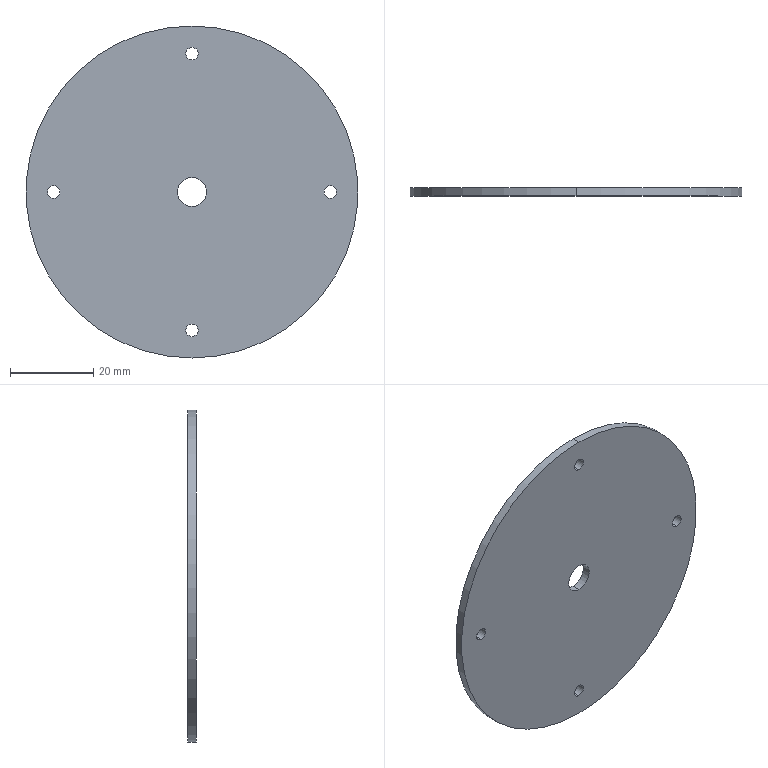Part | SolidWorks | features Cut 2, Extrusion 1 | 1 solid | 14 faces | box 80 x 2 x 80 mm | volume 9920 mm3 | cylinder 12 | plane 2 | commonest cylinder face diameters 3 x8 7 x2 80 x2
STEP:
#1=CARTESIAN_POINT('',(0.,0.,-34.839));
#2=VERTEX_POINT('',#1);
#3=CARTESIAN_POINT('',(0.,0.,-31.839));
#4=VERTEX_POINT('',#3);
#5=CARTESIAN_POINT('',(0.,0.,-33.339));
#6=DIRECTION('',(0.,1.,0.));
#7=DIRECTION('',(0.,0.,1.));
#8=AXIS2_PLACEMENT_3D('',#5,#6,#7);
#9=CIRCLE('',#8,1.5);
#10=EDGE_CURVE('',#2,#4,#9,.T.);
#11=ORIENTED_EDGE('',*,*,#10,.F.);
#12=CARTESIAN_POINT('',(0.,2.,-34.839));
#13=VERTEX_POINT('',#12);
#14=CARTESIAN_POINT('',(0.,-43.,-34.839));
#15=DIRECTION('',(0.,1.,0.));
#16=VECTOR('',#15,1000.);
#17=LINE('',#14,#16);
#18=EDGE_CURVE('',#2,#13,#17,.T.);
#19=ORIENTED_EDGE('',*,*,#18,.T.);
#20=CARTESIAN_POINT('',(0.,2.,-31.839));
#21=VERTEX_POINT('',#20);
#22=CARTESIAN_POINT('',(0.,2.,-33.339));
#23=DIRECTION('',(0.,1.,0.));
#24=DIRECTION('',(0.,0.,1.));
#25=AXIS2_PLACEMENT_3D('',#22,#23,#24);
#26=CIRCLE('',#25,1.5);
#27=EDGE_CURVE('',#13,#21,#26,.T.);
#28=ORIENTED_EDGE('',*,*,#27,.T.);
#29=CARTESIAN_POINT('',(0.,-43.,-31.839));
#30=DIRECTION('',(0.,1.,0.));
#31=VECTOR('',#30,1000.);
#32=LINE('',#29,#31);
#33=EDGE_CURVE('',#4,#21,#32,.T.);
#34=ORIENTED_EDGE('',*,*,#33,.F.);
#35=EDGE_LOOP('',(#11,#19,#28,#34));
#36=FACE_OUTER_BOUND('',#35,.T.);
#37=CARTESIAN_POINT('',(0.,-43.,-33.339));
#38=DIRECTION('',(0.,1.,0.));
#39=DIRECTION('',(0.,0.,1.));
#40=AXIS2_PLACEMENT_3D('',#37,#38,#39);
#41=CYLINDRICAL_SURFACE('',#40,1.5);
#42=ADVANCED_FACE('',(#36),#41,.F.);
#43=CARTESIAN_POINT('',(33.339,0.,-1.5));
#44=VERTEX_POINT('',#43);
#45=CARTESIAN_POINT('',(33.339,0.,1.5));
#46=VERTEX_POINT('',#45);
#47=CARTESIAN_POINT('',(33.339,0.,0.));
#48=DIRECTION('',(0.,1.,0.));
#49=DIRECTION('',(0.,0.,1.));
#50=AXIS2_PLACEMENT_3D('',#47,#48,#49);
#51=CIRCLE('',#50,1.5);
#52=EDGE_CURVE('',#44,#46,#51,.T.);
#53=ORIENTED_EDGE('',*,*,#52,.F.);
#54=CARTESIAN_POINT('',(33.339,2.,-1.5));
#55=VERTEX_POINT('',#54);
#56=CARTESIAN_POINT('',(33.339,-43.,-1.5));
#57=DIRECTION('',(0.,1.,0.));
#58=VECTOR('',#57,1000.);
#59=LINE('',#56,#58);
#60=EDGE_CURVE('',#44,#55,#59,.T.);
#61=ORIENTED_EDGE('',*,*,#60,.T.);
#62=CARTESIAN_POINT('',(33.339,2.,1.5));
#63=VERTEX_POINT('',#62);
#64=CARTESIAN_POINT('',(33.339,2.,0.));
#65=DIRECTION('',(0.,1.,0.));
#66=DIRECTION('',(0.,0.,1.));
#67=AXIS2_PLACEMENT_3D('',#64,#65,#66);
#68=CIRCLE('',#67,1.5);
#69=EDGE_CURVE('',#55,#63,#68,.T.);
#70=ORIENTED_EDGE('',*,*,#69,.T.);
#71=CARTESIAN_POINT('',(33.339,-43.,1.5));
#72=DIRECTION('',(0.,1.,0.));
#73=VECTOR('',#72,1000.);
#74=LINE('',#71,#73);
#75=EDGE_CURVE('',#46,#63,#74,.T.);
#76=ORIENTED_EDGE('',*,*,#75,.F.);
#77=EDGE_LOOP('',(#53,#61,#70,#76));
#78=FACE_OUTER_BOUND('',#77,.T.);
#79=CARTESIAN_POINT('',(33.339,-43.,0.));
#80=DIRECTION('',(0.,1.,0.));
#81=DIRECTION('',(0.,0.,1.));
#82=AXIS2_PLACEMENT_3D('',#79,#80,#81);
#83=CYLINDRICAL_SURFACE('',#82,1.5);
#84=ADVANCED_FACE('',(#78),#83,.F.);
#85=CARTESIAN_POINT('',(0.,0.,31.839));
#86=VERTEX_POINT('',#85);
#87=CARTESIAN_POINT('',(0.,0.,34.839));
#88=VERTEX_POINT('',#87);
#89=CARTESIAN_POINT('',(0.,0.,33.339));
#90=DIRECTION('',(0.,1.,0.));
#91=DIRECTION('',(0.,0.,1.));
#92=AXIS2_PLACEMENT_3D('',#89,#90,#91);
#93=CIRCLE('',#92,1.5);
#94=EDGE_CURVE('',#86,#88,#93,.T.);
#95=ORIENTED_EDGE('',*,*,#94,.F.);
#96=CARTESIAN_POINT('',(0.,2.,31.839));
#97=VERTEX_POINT('',#96);
#98=CARTESIAN_POINT('',(0.,-43.,31.839));
#99=DIRECTION('',(0.,1.,0.));
#100=VECTOR('',#99,1000.);
#101=LINE('',#98,#100);
#102=EDGE_CURVE('',#86,#97,#101,.T.);
#103=ORIENTED_EDGE('',*,*,#102,.T.);
#104=CARTESIAN_POINT('',(0.,2.,34.839));
#105=VERTEX_POINT('',#104);
#106=CARTESIAN_POINT('',(0.,2.,33.339));
#107=DIRECTION('',(0.,1.,0.));
#108=DIRECTION('',(0.,0.,1.));
#109=AXIS2_PLACEMENT_3D('',#106,#107,#108);
#110=CIRCLE('',#109,1.5);
#111=EDGE_CURVE('',#97,#105,#110,.T.);
#112=ORIENTED_EDGE('',*,*,#111,.T.);
#113=CARTESIAN_POINT('',(0.,-43.,34.839));
#114=DIRECTION('',(0.,1.,0.));
#115=VECTOR('',#114,1000.);
#116=LINE('',#113,#115);
#117=EDGE_CURVE('',#88,#105,#116,.T.);
#118=ORIENTED_EDGE('',*,*,#117,.F.);
#119=EDGE_LOOP('',(#95,#103,#112,#118));
#120=FACE_OUTER_BOUND('',#119,.T.);
#121=CARTESIAN_POINT('',(0.,-43.,33.339));
#122=DIRECTION('',(0.,1.,0.));
#123=DIRECTION('',(0.,0.,1.));
#124=AXIS2_PLACEMENT_3D('',#121,#122,#123);
#125=CYLINDRICAL_SURFACE('',#124,1.5);
#126=ADVANCED_FACE('',(#120),#125,.F.);
#127=CARTESIAN_POINT('',(-33.339,0.,-1.5));
#128=VERTEX_POINT('',#127);
#129=CARTESIAN_POINT('',(-33.339,0.,1.5));
#130=VERTEX_POINT('',#129);
#131=CARTESIAN_POINT('',(-33.339,0.,0.));
#132=DIRECTION('',(0.,1.,0.));
#133=DIRECTION('',(0.,0.,1.));
#134=AXIS2_PLACEMENT_3D('',#131,#132,#133);
#135=CIRCLE('',#134,1.5);
#136=EDGE_CURVE('',#128,#130,#135,.T.);
#137=ORIENTED_EDGE('',*,*,#136,.F.);
#138=CARTESIAN_POINT('',(-33.339,2.,-1.5));
#139=VERTEX_POINT('',#138);
#140=CARTESIAN_POINT('',(-33.339,-43.,-1.5));
#141=DIRECTION('',(0.,1.,0.));
#142=VECTOR('',#141,1000.);
#143=LINE('',#140,#142);
#144=EDGE_CURVE('',#128,#139,#143,.T.);
#145=ORIENTED_EDGE('',*,*,#144,.T.);
#146=CARTESIAN_POINT('',(-33.339,2.,1.5));
#147=VERTEX_POINT('',#146);
#148=CARTESIAN_POINT('',(-33.339,2.,0.));
#149=DIRECTION('',(0.,1.,0.));
#150=DIRECTION('',(0.,0.,1.));
#151=AXIS2_PLACEMENT_3D('',#148,#149,#150);
#152=CIRCLE('',#151,1.5);
#153=EDGE_CURVE('',#139,#147,#152,.T.);
#154=ORIENTED_EDGE('',*,*,#153,.T.);
#155=CARTESIAN_POINT('',(-33.339,-43.,1.5));
#156=DIRECTION('',(0.,1.,0.));
#157=VECTOR('',#156,1000.);
#158=LINE('',#155,#157);
#159=EDGE_CURVE('',#130,#147,#158,.T.);
#160=ORIENTED_EDGE('',*,*,#159,.F.);
#161=EDGE_LOOP('',(#137,#145,#154,#160));
#162=FACE_OUTER_BOUND('',#161,.T.);
#163=CARTESIAN_POINT('',(-33.339,-43.,0.));
#164=DIRECTION('',(0.,1.,0.));
#165=DIRECTION('',(0.,0.,1.));
#166=AXIS2_PLACEMENT_3D('',#163,#164,#165);
#167=CYLINDRICAL_SURFACE('',#166,1.5);
#168=ADVANCED_FACE('',(#162),#167,.F.);
#169=CARTESIAN_POINT('',(0.,2.,-3.5));
#170=VERTEX_POINT('',#169);
#171=CARTESIAN_POINT('',(0.,2.,3.5));
#172=VERTEX_POINT('',#171);
#173=CARTESIAN_POINT('',(0.,2.,0.));
#174=DIRECTION('',(0.,1.,0.));
#175=DIRECTION('',(0.,0.,1.));
#176=AXIS2_PLACEMENT_3D('',#173,#174,#175);
#177=CIRCLE('',#176,3.5);
#178=EDGE_CURVE('',#170,#172,#177,.T.);
#179=ORIENTED_EDGE('',*,*,#178,.T.);
#180=CARTESIAN_POINT('',(0.,0.,3.5));
#181=VERTEX_POINT('',#180);
#182=CARTESIAN_POINT('',(0.,52.,3.5));
#183=DIRECTION('',(0.,-1.,0.));
#184=VECTOR('',#183,1000.);
#185=LINE('',#182,#184);
#186=EDGE_CURVE('',#172,#181,#185,.T.);
#187=ORIENTED_EDGE('',*,*,#186,.T.);
#188=CARTESIAN_POINT('',(0.,0.,-3.5));
#189=VERTEX_POINT('',#188);
#190=CARTESIAN_POINT('',(0.,0.,0.));
#191=DIRECTION('',(0.,-1.,0.));
#192=DIRECTION('',(0.,0.,-1.));
#193=AXIS2_PLACEMENT_3D('',#190,#191,#192);
#194=CIRCLE('',#193,3.5);
#195=EDGE_CURVE('',#181,#189,#194,.T.);
#196=ORIENTED_EDGE('',*,*,#195,.T.);
#197=CARTESIAN_POINT('',(0.,52.,-3.5));
#198=DIRECTION('',(0.,-1.,0.));
#199=VECTOR('',#198,1000.);
#200=LINE('',#197,#199);
#201=EDGE_CURVE('',#170,#189,#200,.T.);
#202=ORIENTED_EDGE('',*,*,#201,.F.);
#203=EDGE_LOOP('',(#179,#187,#196,#202));
#204=FACE_OUTER_BOUND('',#203,.T.);
#205=CARTESIAN_POINT('',(0.,52.,0.));
#206=DIRECTION('',(0.,-1.,0.));
#207=DIRECTION('',(0.,0.,-1.));
#208=AXIS2_PLACEMENT_3D('',#205,#206,#207);
#209=CYLINDRICAL_SURFACE('',#208,3.5);
#210=ADVANCED_FACE('',(#204),#209,.F.);
#211=CARTESIAN_POINT('',(0.,2.,40.));
#212=VERTEX_POINT('',#211);
#213=CARTESIAN_POINT('',(0.,2.,-40.));
#214=VERTEX_POINT('',#213);
#215=CARTESIAN_POINT('',(0.,2.,0.));
#216=DIRECTION('',(0.,1.,0.));
#217=DIRECTION('',(0.,0.,1.));
#218=AXIS2_PLACEMENT_3D('',#215,#216,#217);
#219=CIRCLE('',#218,40.);
#220=EDGE_CURVE('',#212,#214,#219,.T.);
#221=ORIENTED_EDGE('',*,*,#220,.F.);
#222=CARTESIAN_POINT('',(0.,0.,40.));
#223=VERTEX_POINT('',#222);
#224=CARTESIAN_POINT('',(0.,2.,40.));
#225=DIRECTION('',(0.,-1.,0.));
#226=VECTOR('',#225,1000.);
#227=LINE('',#224,#226);
#228=EDGE_CURVE('',#212,#223,#227,.T.);
#229=ORIENTED_EDGE('',*,*,#228,.T.);
#230=CARTESIAN_POINT('',(0.,0.,-40.));
#231=VERTEX_POINT('',#230);
#232=CARTESIAN_POINT('',(0.,0.,0.));
#233=DIRECTION('',(0.,1.,0.));
#234=DIRECTION('',(0.,0.,1.));
#235=AXIS2_PLACEMENT_3D('',#232,#233,#234);
#236=CIRCLE('',#235,40.);
#237=EDGE_CURVE('',#223,#231,#236,.T.);
#238=ORIENTED_EDGE('',*,*,#237,.T.);
#239=CARTESIAN_POINT('',(0.,2.,-40.));
#240=DIRECTION('',(0.,-1.,0.));
#241=VECTOR('',#240,1000.);
#242=LINE('',#239,#241);
#243=EDGE_CURVE('',#214,#231,#242,.T.);
#244=ORIENTED_EDGE('',*,*,#243,.F.);
#245=EDGE_LOOP('',(#221,#229,#238,#244));
#246=FACE_OUTER_BOUND('',#245,.T.);
#247=CARTESIAN_POINT('',(0.,2.,0.));
#248=DIRECTION('',(0.,-1.,0.));
#249=DIRECTION('',(0.,0.,-1.));
#250=AXIS2_PLACEMENT_3D('',#247,#248,#249);
#251=CYLINDRICAL_SURFACE('',#250,40.);
#252=ADVANCED_FACE('',(#246),#251,.T.);
#253=ORIENTED_EDGE('',*,*,#228,.F.);
#254=CARTESIAN_POINT('',(0.,2.,0.));
#255=DIRECTION('',(0.,1.,0.));
#256=DIRECTION('',(0.,0.,1.));
#257=AXIS2_PLACEMENT_3D('',#254,#255,#256);
#258=CIRCLE('',#257,40.);
#259=EDGE_CURVE('',#214,#212,#258,.T.);
#260=ORIENTED_EDGE('',*,*,#259,.F.);
#261=ORIENTED_EDGE('',*,*,#243,.T.);
#262=CARTESIAN_POINT('',(0.,0.,0.));
#263=DIRECTION('',(0.,1.,0.));
#264=DIRECTION('',(0.,0.,1.));
#265=AXIS2_PLACEMENT_3D('',#262,#263,#264);
#266=CIRCLE('',#265,40.);
#267=EDGE_CURVE('',#231,#223,#266,.T.);
#268=ORIENTED_EDGE('',*,*,#267,.T.);
#269=EDGE_LOOP('',(#253,#260,#261,#268));
#270=FACE_OUTER_BOUND('',#269,.T.);
#271=CARTESIAN_POINT('',(0.,2.,0.));
#272=DIRECTION('',(0.,-1.,0.));
#273=DIRECTION('',(0.,0.,-1.));
#274=AXIS2_PLACEMENT_3D('',#271,#272,#273);
#275=CYLINDRICAL_SURFACE('',#274,40.);
#276=ADVANCED_FACE('',(#270),#275,.T.);
#277=CARTESIAN_POINT('',(0.,2.,-33.339));
#278=DIRECTION('',(0.,1.,0.));
#279=DIRECTION('',(0.,0.,1.));
#280=AXIS2_PLACEMENT_3D('',#277,#278,#279);
#281=CIRCLE('',#280,1.5);
#282=EDGE_CURVE('',#21,#13,#281,.T.);
#283=ORIENTED_EDGE('',*,*,#282,.F.);
#284=ORIENTED_EDGE('',*,*,#27,.F.);
#285=EDGE_LOOP('',(#283,#284));
#286=FACE_BOUND('',#285,.T.);
#287=CARTESIAN_POINT('',(33.339,2.,0.));
#288=DIRECTION('',(0.,1.,0.));
#289=DIRECTION('',(0.,0.,1.));
#290=AXIS2_PLACEMENT_3D('',#287,#288,#289);
#291=CIRCLE('',#290,1.5);
#292=EDGE_CURVE('',#63,#55,#291,.T.);
#293=ORIENTED_EDGE('',*,*,#292,.F.);
#294=ORIENTED_EDGE('',*,*,#69,.F.);
#295=EDGE_LOOP('',(#293,#294));
#296=FACE_BOUND('',#295,.T.);
#297=CARTESIAN_POINT('',(0.,2.,33.339));
#298=DIRECTION('',(0.,1.,0.));
#299=DIRECTION('',(0.,0.,1.));
#300=AXIS2_PLACEMENT_3D('',#297,#298,#299);
#301=CIRCLE('',#300,1.5);
#302=EDGE_CURVE('',#105,#97,#301,.T.);
#303=ORIENTED_EDGE('',*,*,#302,.F.);
#304=ORIENTED_EDGE('',*,*,#111,.F.);
#305=EDGE_LOOP('',(#303,#304));
#306=FACE_BOUND('',#305,.T.);
#307=CARTESIAN_POINT('',(-33.339,2.,0.));
#308=DIRECTION('',(0.,1.,0.));
#309=DIRECTION('',(0.,0.,1.));
#310=AXIS2_PLACEMENT_3D('',#307,#308,#309);
#311=CIRCLE('',#310,1.5);
#312=EDGE_CURVE('',#147,#139,#311,.T.);
#313=ORIENTED_EDGE('',*,*,#312,.F.);
#314=ORIENTED_EDGE('',*,*,#153,.F.);
#315=EDGE_LOOP('',(#313,#314));
#316=FACE_BOUND('',#315,.T.);
#317=ORIENTED_EDGE('',*,*,#178,.F.);
#318=CARTESIAN_POINT('',(0.,2.,0.));
#319=DIRECTION('',(0.,1.,0.));
#320=DIRECTION('',(0.,0.,1.));
#321=AXIS2_PLACEMENT_3D('',#318,#319,#320);
#322=CIRCLE('',#321,3.5);
#323=EDGE_CURVE('',#172,#170,#322,.T.);
#324=ORIENTED_EDGE('',*,*,#323,.F.);
#325=EDGE_LOOP('',(#317,#324));
#326=FACE_BOUND('',#325,.T.);
#327=ORIENTED_EDGE('',*,*,#259,.T.);
#328=ORIENTED_EDGE('',*,*,#220,.T.);
#329=EDGE_LOOP('',(#327,#328));
#330=FACE_OUTER_BOUND('',#329,.T.);
#331=CARTESIAN_POINT('',(0.,2.,0.));
#332=DIRECTION('',(0.,1.,0.));
#333=DIRECTION('',(0.,0.,1.));
#334=AXIS2_PLACEMENT_3D('',#331,#332,#333);
#335=PLANE('',#334);
#336=ADVANCED_FACE('',(#286,#296,#306,#316,#326,#330),#335,.T.);
#337=CARTESIAN_POINT('',(0.,0.,-33.339));
#338=DIRECTION('',(0.,1.,0.));
#339=DIRECTION('',(0.,0.,1.));
#340=AXIS2_PLACEMENT_3D('',#337,#338,#339);
#341=CIRCLE('',#340,1.5);
#342=EDGE_CURVE('',#4,#2,#341,.T.);
#343=ORIENTED_EDGE('',*,*,#342,.T.);
#344=ORIENTED_EDGE('',*,*,#10,.T.);
#345=EDGE_LOOP('',(#343,#344));
#346=FACE_BOUND('',#345,.T.);
#347=CARTESIAN_POINT('',(33.339,0.,0.));
#348=DIRECTION('',(0.,1.,0.));
#349=DIRECTION('',(0.,0.,1.));
#350=AXIS2_PLACEMENT_3D('',#347,#348,#349);
#351=CIRCLE('',#350,1.5);
#352=EDGE_CURVE('',#46,#44,#351,.T.);
#353=ORIENTED_EDGE('',*,*,#352,.T.);
#354=ORIENTED_EDGE('',*,*,#52,.T.);
#355=EDGE_LOOP('',(#353,#354));
#356=FACE_BOUND('',#355,.T.);
#357=CARTESIAN_POINT('',(0.,0.,33.339));
#358=DIRECTION('',(0.,1.,0.));
#359=DIRECTION('',(0.,0.,1.));
#360=AXIS2_PLACEMENT_3D('',#357,#358,#359);
#361=CIRCLE('',#360,1.5);
#362=EDGE_CURVE('',#88,#86,#361,.T.);
#363=ORIENTED_EDGE('',*,*,#362,.T.);
#364=ORIENTED_EDGE('',*,*,#94,.T.);
#365=EDGE_LOOP('',(#363,#364));
#366=FACE_BOUND('',#365,.T.);
#367=CARTESIAN_POINT('',(-33.339,0.,0.));
#368=DIRECTION('',(0.,1.,0.));
#369=DIRECTION('',(0.,0.,1.));
#370=AXIS2_PLACEMENT_3D('',#367,#368,#369);
#371=CIRCLE('',#370,1.5);
#372=EDGE_CURVE('',#130,#128,#371,.T.);
#373=ORIENTED_EDGE('',*,*,#372,.T.);
#374=ORIENTED_EDGE('',*,*,#136,.T.);
#375=EDGE_LOOP('',(#373,#374));
#376=FACE_BOUND('',#375,.T.);
#377=CARTESIAN_POINT('',(0.,0.,0.));
#378=DIRECTION('',(0.,-1.,0.));
#379=DIRECTION('',(0.,0.,-1.));
#380=AXIS2_PLACEMENT_3D('',#377,#378,#379);
#381=CIRCLE('',#380,3.5);
#382=EDGE_CURVE('',#189,#181,#381,.T.);
#383=ORIENTED_EDGE('',*,*,#382,.F.);
#384=ORIENTED_EDGE('',*,*,#195,.F.);
#385=EDGE_LOOP('',(#383,#384));
#386=FACE_BOUND('',#385,.T.);
#387=ORIENTED_EDGE('',*,*,#267,.F.);
#388=ORIENTED_EDGE('',*,*,#237,.F.);
#389=EDGE_LOOP('',(#387,#388));
#390=FACE_OUTER_BOUND('',#389,.T.);
#391=CARTESIAN_POINT('',(0.,0.,0.));
#392=DIRECTION('',(0.,1.,0.));
#393=DIRECTION('',(0.,0.,1.));
#394=AXIS2_PLACEMENT_3D('',#391,#392,#393);
#395=PLANE('',#394);
#396=ADVANCED_FACE('',(#346,#356,#366,#376,#386,#390),#395,.F.);
#397=ORIENTED_EDGE('',*,*,#186,.F.);
#398=ORIENTED_EDGE('',*,*,#323,.T.);
#399=ORIENTED_EDGE('',*,*,#201,.T.);
#400=ORIENTED_EDGE('',*,*,#382,.T.);
#401=EDGE_LOOP('',(#397,#398,#399,#400));
#402=FACE_OUTER_BOUND('',#401,.T.);
#403=CARTESIAN_POINT('',(0.,52.,0.));
#404=DIRECTION('',(0.,-1.,0.));
#405=DIRECTION('',(0.,0.,-1.));
#406=AXIS2_PLACEMENT_3D('',#403,#404,#405);
#407=CYLINDRICAL_SURFACE('',#406,3.5);
#408=ADVANCED_FACE('',(#402),#407,.F.);
#409=ORIENTED_EDGE('',*,*,#144,.F.);
#410=ORIENTED_EDGE('',*,*,#372,.F.);
#411=ORIENTED_EDGE('',*,*,#159,.T.);
#412=ORIENTED_EDGE('',*,*,#312,.T.);
#413=EDGE_LOOP('',(#409,#410,#411,#412));
#414=FACE_OUTER_BOUND('',#413,.T.);
#415=CARTESIAN_POINT('',(-33.339,-43.,0.));
#416=DIRECTION('',(0.,1.,0.));
#417=DIRECTION('',(0.,0.,1.));
#418=AXIS2_PLACEMENT_3D('',#415,#416,#417);
#419=CYLINDRICAL_SURFACE('',#418,1.5);
#420=ADVANCED_FACE('',(#414),#419,.F.);
#421=ORIENTED_EDGE('',*,*,#102,.F.);
#422=ORIENTED_EDGE('',*,*,#362,.F.);
#423=ORIENTED_EDGE('',*,*,#117,.T.);
#424=ORIENTED_EDGE('',*,*,#302,.T.);
#425=EDGE_LOOP('',(#421,#422,#423,#424));
#426=FACE_OUTER_BOUND('',#425,.T.);
#427=CARTESIAN_POINT('',(0.,-43.,33.339));
#428=DIRECTION('',(0.,1.,0.));
#429=DIRECTION('',(0.,0.,1.));
#430=AXIS2_PLACEMENT_3D('',#427,#428,#429);
#431=CYLINDRICAL_SURFACE('',#430,1.5);
#432=ADVANCED_FACE('',(#426),#431,.F.);
#433=ORIENTED_EDGE('',*,*,#60,.F.);
#434=ORIENTED_EDGE('',*,*,#352,.F.);
#435=ORIENTED_EDGE('',*,*,#75,.T.);
#436=ORIENTED_EDGE('',*,*,#292,.T.);
#437=EDGE_LOOP('',(#433,#434,#435,#436));
#438=FACE_OUTER_BOUND('',#437,.T.);
#439=CARTESIAN_POINT('',(33.339,-43.,0.));
#440=DIRECTION('',(0.,1.,0.));
#441=DIRECTION('',(0.,0.,1.));
#442=AXIS2_PLACEMENT_3D('',#439,#440,#441);
#443=CYLINDRICAL_SURFACE('',#442,1.5);
#444=ADVANCED_FACE('',(#438),#443,.F.);
#445=ORIENTED_EDGE('',*,*,#18,.F.);
#446=ORIENTED_EDGE('',*,*,#342,.F.);
#447=ORIENTED_EDGE('',*,*,#33,.T.);
#448=ORIENTED_EDGE('',*,*,#282,.T.);
#449=EDGE_LOOP('',(#445,#446,#447,#448));
#450=FACE_OUTER_BOUND('',#449,.T.);
#451=CARTESIAN_POINT('',(0.,-43.,-33.339));
#452=DIRECTION('',(0.,1.,0.));
#453=DIRECTION('',(0.,0.,1.));
#454=AXIS2_PLACEMENT_3D('',#451,#452,#453);
#455=CYLINDRICAL_SURFACE('',#454,1.5);
#456=ADVANCED_FACE('',(#450),#455,.F.);
#457=CLOSED_SHELL('',(#42,#84,#126,#168,#210,#252,#276,#336,#396,#408,#420,#432,#444,#456));
#458=MANIFOLD_SOLID_BREP('',#457);
#459=CARTESIAN_POINT('',(0.,0.,0.));
#460=DIRECTION('',(0.,0.,1.));
#461=DIRECTION('',(1.,0.,0.));
#462=AXIS2_PLACEMENT_3D('',#459,#460,#461);
#463=(LENGTH_UNIT()NAMED_UNIT(*)SI_UNIT(.MILLI.,.METRE.));
#464=UNCERTAINTY_MEASURE_WITH_UNIT(LENGTH_MEASURE(0.00001),#463,'','');
#465=(NAMED_UNIT(*)PLANE_ANGLE_UNIT()SI_UNIT($,.RADIAN.));
#466=(NAMED_UNIT(*)SI_UNIT($,.STERADIAN.)SOLID_ANGLE_UNIT());
#467=(GEOMETRIC_REPRESENTATION_CONTEXT(3)GLOBAL_UNCERTAINTY_ASSIGNED_CONTEXT((#464))GLOBAL_UNIT_ASSIGNED_CONTEXT((#463,#465,#466))REPRESENTATION_CONTEXT('',''));
#468=ADVANCED_BREP_SHAPE_REPRESENTATION('',(#458,#462),#467);